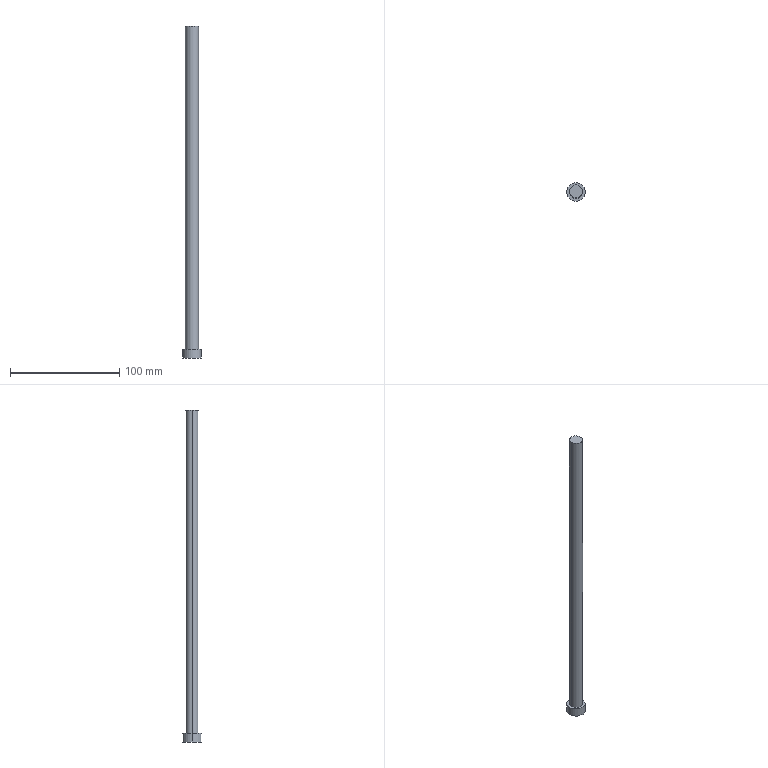Part | Creo | 1 solid | 7 faces | box 17 x 17 x 304.541 mm | volume 35354 mm3 | cylinder 4 | plane 3 | commonest cylinder face diameters 12 x2 17 x2
STEP:
#1=CARTESIAN_POINT('',(0.,0.,0.));
#2=DIRECTION('',(0.,0.,1.));
#3=DIRECTION('',(1.,0.,0.));
#4=AXIS2_PLACEMENT_3D('',#1,#2,#3);
#5=CARTESIAN_POINT('',(-129.641,96.984,-33.901));
#6=VERTEX_POINT('',#5);
#7=CARTESIAN_POINT('',(-141.641,96.984,-33.901));
#8=VERTEX_POINT('',#7);
#9=CARTESIAN_POINT('',(-135.641,96.984,-33.901));
#10=DIRECTION('',(0.,0.,1.));
#11=DIRECTION('',(1.,0.,0.));
#12=AXIS2_PLACEMENT_3D('',#9,#10,#11);
#13=CIRCLE('',#12,6.);
#14=EDGE_CURVE('',#6,#8,#13,.T.);
#15=ORIENTED_EDGE('',*,*,#14,.F.);
#16=CARTESIAN_POINT('',(-135.641,96.984,-33.901));
#17=DIRECTION('',(0.,0.,1.));
#18=DIRECTION('',(-1.,0.,0.));
#19=AXIS2_PLACEMENT_3D('',#16,#17,#18);
#20=CIRCLE('',#19,6.);
#21=EDGE_CURVE('',#8,#6,#20,.T.);
#22=ORIENTED_EDGE('',*,*,#21,.F.);
#23=EDGE_LOOP('',(#15,#22));
#24=FACE_OUTER_BOUND('',#23,.F.);
#25=CARTESIAN_POINT('',(-135.641,96.984,-33.901));
#26=DIRECTION('',(0.,0.,1.));
#27=DIRECTION('',(1.,0.,0.));
#28=AXIS2_PLACEMENT_3D('',#25,#26,#27);
#29=PLANE('',#28);
#30=ADVANCED_FACE('',(#24),#29,.T.);
#31=CARTESIAN_POINT('',(-141.641,96.984,-330.441));
#32=VERTEX_POINT('',#31);
#33=CARTESIAN_POINT('',(-129.641,96.984,-330.441));
#34=VERTEX_POINT('',#33);
#35=CARTESIAN_POINT('',(-135.641,96.984,-330.441));
#36=DIRECTION('',(0.,0.,-1.));
#37=DIRECTION('',(-1.,0.,0.));
#38=AXIS2_PLACEMENT_3D('',#35,#36,#37);
#39=CIRCLE('',#38,6.);
#40=EDGE_CURVE('',#32,#34,#39,.T.);
#41=ORIENTED_EDGE('',*,*,#40,.T.);
#42=CARTESIAN_POINT('',(-129.641,96.984,-33.901));
#43=DIRECTION('',(0.,0.,-1.));
#44=VECTOR('',#43,296.541);
#45=LINE('',#42,#44);
#46=EDGE_CURVE('',#6,#34,#45,.T.);
#47=ORIENTED_EDGE('',*,*,#46,.F.);
#48=ORIENTED_EDGE('',*,*,#14,.T.);
#49=CARTESIAN_POINT('',(-141.641,96.984,-33.901));
#50=DIRECTION('',(0.,0.,-1.));
#51=VECTOR('',#50,296.541);
#52=LINE('',#49,#51);
#53=EDGE_CURVE('',#8,#32,#52,.T.);
#54=ORIENTED_EDGE('',*,*,#53,.T.);
#55=EDGE_LOOP('',(#41,#47,#48,#54));
#56=FACE_OUTER_BOUND('',#55,.F.);
#57=CARTESIAN_POINT('',(-135.641,96.984,-33.901));
#58=DIRECTION('',(0.,0.,-1.));
#59=DIRECTION('',(-1.,0.,0.));
#60=AXIS2_PLACEMENT_3D('',#57,#58,#59);
#61=CYLINDRICAL_SURFACE('',#60,6.);
#62=ADVANCED_FACE('',(#56),#61,.T.);
#63=CARTESIAN_POINT('',(-144.141,96.984,-330.441));
#64=VERTEX_POINT('',#63);
#65=CARTESIAN_POINT('',(-127.141,96.984,-330.441));
#66=VERTEX_POINT('',#65);
#67=CARTESIAN_POINT('',(-135.641,96.984,-330.441));
#68=DIRECTION('',(0.,0.,1.));
#69=DIRECTION('',(-1.,0.,0.));
#70=AXIS2_PLACEMENT_3D('',#67,#68,#69);
#71=CIRCLE('',#70,8.5);
#72=EDGE_CURVE('',#64,#66,#71,.T.);
#73=ORIENTED_EDGE('',*,*,#72,.F.);
#74=CARTESIAN_POINT('',(-135.641,96.984,-330.441));
#75=DIRECTION('',(0.,0.,1.));
#76=DIRECTION('',(1.,0.,0.));
#77=AXIS2_PLACEMENT_3D('',#74,#75,#76);
#78=CIRCLE('',#77,8.5);
#79=EDGE_CURVE('',#66,#64,#78,.T.);
#80=ORIENTED_EDGE('',*,*,#79,.F.);
#81=EDGE_LOOP('',(#73,#80));
#82=FACE_OUTER_BOUND('',#81,.F.);
#83=CARTESIAN_POINT('',(-135.641,96.984,-330.441));
#84=DIRECTION('',(0.,0.,-1.));
#85=DIRECTION('',(1.,0.,0.));
#86=AXIS2_PLACEMENT_3D('',#83,#84,#85);
#87=CIRCLE('',#86,6.);
#88=EDGE_CURVE('',#34,#32,#87,.T.);
#89=ORIENTED_EDGE('',*,*,#88,.F.);
#90=ORIENTED_EDGE('',*,*,#40,.F.);
#91=EDGE_LOOP('',(#89,#90));
#92=FACE_BOUND('',#91,.F.);
#93=CARTESIAN_POINT('',(-135.641,96.984,-330.441));
#94=DIRECTION('',(0.,0.,1.));
#95=DIRECTION('',(1.,0.,0.));
#96=AXIS2_PLACEMENT_3D('',#93,#94,#95);
#97=PLANE('',#96);
#98=ADVANCED_FACE('',(#82,#92),#97,.T.);
#99=ORIENTED_EDGE('',*,*,#72,.T.);
#100=CARTESIAN_POINT('',(-127.141,96.984,-338.441));
#101=VERTEX_POINT('',#100);
#102=CARTESIAN_POINT('',(-127.141,96.984,-330.441));
#103=DIRECTION('',(0.,0.,-1.));
#104=VECTOR('',#103,8.);
#105=LINE('',#102,#104);
#106=EDGE_CURVE('',#66,#101,#105,.T.);
#107=ORIENTED_EDGE('',*,*,#106,.T.);
#108=CARTESIAN_POINT('',(-144.141,96.984,-338.441));
#109=VERTEX_POINT('',#108);
#110=CARTESIAN_POINT('',(-135.641,96.984,-338.441));
#111=DIRECTION('',(0.,0.,-1.));
#112=DIRECTION('',(1.,0.,0.));
#113=AXIS2_PLACEMENT_3D('',#110,#111,#112);
#114=CIRCLE('',#113,8.5);
#115=EDGE_CURVE('',#101,#109,#114,.T.);
#116=ORIENTED_EDGE('',*,*,#115,.T.);
#117=CARTESIAN_POINT('',(-144.141,96.984,-330.441));
#118=DIRECTION('',(0.,0.,-1.));
#119=VECTOR('',#118,8.);
#120=LINE('',#117,#119);
#121=EDGE_CURVE('',#64,#109,#120,.T.);
#122=ORIENTED_EDGE('',*,*,#121,.F.);
#123=EDGE_LOOP('',(#99,#107,#116,#122));
#124=FACE_OUTER_BOUND('',#123,.F.);
#125=CARTESIAN_POINT('',(-135.641,96.984,-330.441));
#126=DIRECTION('',(0.,0.,-1.));
#127=DIRECTION('',(-1.,0.,0.));
#128=AXIS2_PLACEMENT_3D('',#125,#126,#127);
#129=CYLINDRICAL_SURFACE('',#128,8.5);
#130=ADVANCED_FACE('',(#124),#129,.T.);
#131=ORIENTED_EDGE('',*,*,#79,.T.);
#132=ORIENTED_EDGE('',*,*,#121,.T.);
#133=CARTESIAN_POINT('',(-135.641,96.984,-338.441));
#134=DIRECTION('',(0.,0.,-1.));
#135=DIRECTION('',(-1.,0.,0.));
#136=AXIS2_PLACEMENT_3D('',#133,#134,#135);
#137=CIRCLE('',#136,8.5);
#138=EDGE_CURVE('',#109,#101,#137,.T.);
#139=ORIENTED_EDGE('',*,*,#138,.T.);
#140=ORIENTED_EDGE('',*,*,#106,.F.);
#141=EDGE_LOOP('',(#131,#132,#139,#140));
#142=FACE_OUTER_BOUND('',#141,.F.);
#143=CARTESIAN_POINT('',(-135.641,96.984,-330.441));
#144=DIRECTION('',(0.,0.,-1.));
#145=DIRECTION('',(-1.,0.,0.));
#146=AXIS2_PLACEMENT_3D('',#143,#144,#145);
#147=CYLINDRICAL_SURFACE('',#146,8.5);
#148=ADVANCED_FACE('',(#142),#147,.T.);
#149=ORIENTED_EDGE('',*,*,#138,.F.);
#150=ORIENTED_EDGE('',*,*,#115,.F.);
#151=EDGE_LOOP('',(#149,#150));
#152=FACE_OUTER_BOUND('',#151,.F.);
#153=CARTESIAN_POINT('',(-453.493,128.373,-338.441));
#154=DIRECTION('',(0.,0.,-1.));
#155=DIRECTION('',(-1.,0.,0.));
#156=AXIS2_PLACEMENT_3D('',#153,#154,#155);
#157=PLANE('',#156);
#158=ADVANCED_FACE('',(#152),#157,.T.);
#159=ORIENTED_EDGE('',*,*,#88,.T.);
#160=ORIENTED_EDGE('',*,*,#53,.F.);
#161=ORIENTED_EDGE('',*,*,#21,.T.);
#162=ORIENTED_EDGE('',*,*,#46,.T.);
#163=EDGE_LOOP('',(#159,#160,#161,#162));
#164=FACE_OUTER_BOUND('',#163,.F.);
#165=CARTESIAN_POINT('',(-135.641,96.984,-33.901));
#166=DIRECTION('',(0.,0.,-1.));
#167=DIRECTION('',(-1.,0.,0.));
#168=AXIS2_PLACEMENT_3D('',#165,#166,#167);
#169=CYLINDRICAL_SURFACE('',#168,6.);
#170=ADVANCED_FACE('',(#164),#169,.T.);
#171=CLOSED_SHELL('',(#30,#62,#98,#130,#148,#158,#170));
#172=MANIFOLD_SOLID_BREP('',#171);
#173=(LENGTH_UNIT()NAMED_UNIT(*)SI_UNIT(.MILLI.,.METRE.));
#174=UNCERTAINTY_MEASURE_WITH_UNIT(LENGTH_MEASURE(0.03055),#173,'','');
#175=(NAMED_UNIT(*)PLANE_ANGLE_UNIT()SI_UNIT($,.RADIAN.));
#176=PLANE_ANGLE_MEASURE_WITH_UNIT(PLANE_ANGLE_MEASURE(0.01745),#175);
#177=(CONVERSION_BASED_UNIT('DEGREE',#176)NAMED_UNIT(*)PLANE_ANGLE_UNIT());
#178=(NAMED_UNIT(*)SI_UNIT($,.STERADIAN.)SOLID_ANGLE_UNIT());
#179=(GEOMETRIC_REPRESENTATION_CONTEXT(3)GLOBAL_UNCERTAINTY_ASSIGNED_CONTEXT((#174))GLOBAL_UNIT_ASSIGNED_CONTEXT((#173,#177,#178))REPRESENTATION_CONTEXT('',''));
#180=ADVANCED_BREP_SHAPE_REPRESENTATION('',(#4,#172),#179);